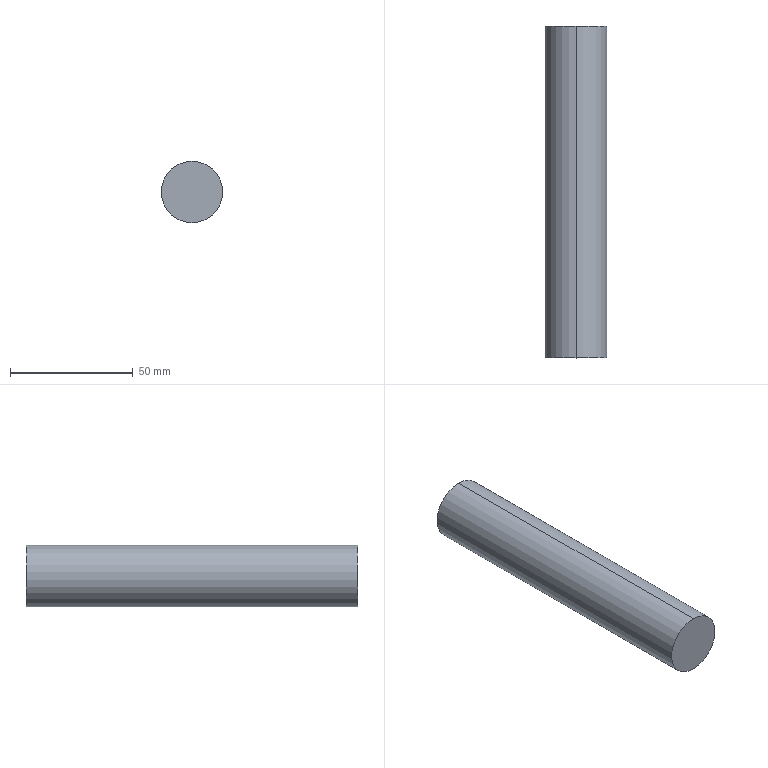Part | 1 solid | 4 faces | box 25 x 135 x 25 mm | volume 66268 mm3 | plane 2 | cylinder 2 | commonest cylinder face diameters 25 x2
STEP:
#1=CARTESIAN_POINT('',(0.,0.,0.));
#2=DIRECTION('',(0.,0.,1.));
#3=DIRECTION('',(1.,0.,0.));
#4=AXIS2_PLACEMENT_3D('',#1,#2,#3);
#5=CARTESIAN_POINT('',(-239.028,-100.5,-288.05));
#6=VERTEX_POINT('',#5);
#7=CARTESIAN_POINT('',(-239.028,-100.5,-313.05));
#8=VERTEX_POINT('',#7);
#9=CARTESIAN_POINT('',(-239.028,-100.5,-300.55));
#10=DIRECTION('',(0.,1.,0.));
#11=DIRECTION('',(0.,0.,-1.));
#12=AXIS2_PLACEMENT_3D('',#9,#10,#11);
#13=CIRCLE('',#12,12.5);
#14=CARTESIAN_POINT('',(-239.028,-100.5,-300.55));
#15=DIRECTION('',(0.,1.,0.));
#16=DIRECTION('',(0.,0.,1.));
#17=AXIS2_PLACEMENT_3D('',#14,#15,#16);
#18=PLANE('',#17);
#19=CARTESIAN_POINT('',(0.,0.));
#20=DIRECTION('',(-1.,0.));
#21=AXIS2_PLACEMENT_2D('',#19,#20);
#22=CIRCLE('',#21,12.5);
#23=(GEOMETRIC_REPRESENTATION_CONTEXT(2)PARAMETRIC_REPRESENTATION_CONTEXT()REPRESENTATION_CONTEXT('',''));
#24=DEFINITIONAL_REPRESENTATION('',(#22),#23);
#25=PCURVE('',#18,#24);
#26=CARTESIAN_POINT('',(-239.028,254.5,-300.55));
#27=DIRECTION('',(0.,-1.,0.));
#28=DIRECTION('',(-1.,0.,0.));
#29=AXIS2_PLACEMENT_3D('',#26,#27,#28);
#30=CYLINDRICAL_SURFACE('',#29,12.5);
#31=CARTESIAN_POINT('',(7.854,355.));
#32=DIRECTION('',(-1.,0.));
#33=VECTOR('',#32,1.);
#34=LINE('',#31,#33);
#35=(GEOMETRIC_REPRESENTATION_CONTEXT(2)PARAMETRIC_REPRESENTATION_CONTEXT()REPRESENTATION_CONTEXT('',''));
#36=DEFINITIONAL_REPRESENTATION('',(#34),#35);
#37=PCURVE('',#30,#36);
#38=SURFACE_CURVE('',#13,(#25,#37),.PCURVE_S1.);
#39=EDGE_CURVE('',#6,#8,#38,.T.);
#40=ORIENTED_EDGE('',*,*,#39,.F.);
#41=CARTESIAN_POINT('',(-239.028,-100.5,-300.55));
#42=DIRECTION('',(0.,1.,0.));
#43=DIRECTION('',(0.,0.,-1.));
#44=AXIS2_PLACEMENT_3D('',#41,#42,#43);
#45=CIRCLE('',#44,12.5);
#46=CARTESIAN_POINT('',(0.,0.));
#47=DIRECTION('',(-1.,0.));
#48=AXIS2_PLACEMENT_2D('',#46,#47);
#49=CIRCLE('',#48,12.5);
#50=(GEOMETRIC_REPRESENTATION_CONTEXT(2)PARAMETRIC_REPRESENTATION_CONTEXT()REPRESENTATION_CONTEXT('',''));
#51=DEFINITIONAL_REPRESENTATION('',(#49),#50);
#52=PCURVE('',#18,#51);
#53=CARTESIAN_POINT('',(-239.028,254.5,-300.55));
#54=DIRECTION('',(0.,-1.,0.));
#55=DIRECTION('',(1.,0.,0.));
#56=AXIS2_PLACEMENT_3D('',#53,#54,#55);
#57=CYLINDRICAL_SURFACE('',#56,12.5);
#58=CARTESIAN_POINT('',(4.712,355.));
#59=DIRECTION('',(-1.,0.));
#60=VECTOR('',#59,1.);
#61=LINE('',#58,#60);
#62=(GEOMETRIC_REPRESENTATION_CONTEXT(2)PARAMETRIC_REPRESENTATION_CONTEXT()REPRESENTATION_CONTEXT('',''));
#63=DEFINITIONAL_REPRESENTATION('',(#61),#62);
#64=PCURVE('',#57,#63);
#65=SURFACE_CURVE('',#45,(#52,#64),.PCURVE_S1.);
#66=EDGE_CURVE('',#8,#6,#65,.T.);
#67=ORIENTED_EDGE('',*,*,#66,.F.);
#68=EDGE_LOOP('',(#40,#67));
#69=FACE_BOUND('',#68,.T.);
#70=ADVANCED_FACE('',(#69),#18,.F.);
#71=CARTESIAN_POINT('',(-239.028,34.5,-288.05));
#72=VERTEX_POINT('',#71);
#73=CARTESIAN_POINT('',(-239.028,34.5,-288.05));
#74=DIRECTION('',(0.,-1.,0.));
#75=VECTOR('',#74,1.);
#76=LINE('',#73,#75);
#77=CARTESIAN_POINT('',(1.571,220.));
#78=DIRECTION('',(0.,1.));
#79=VECTOR('',#78,1.);
#80=LINE('',#77,#79);
#81=(GEOMETRIC_REPRESENTATION_CONTEXT(2)PARAMETRIC_REPRESENTATION_CONTEXT()REPRESENTATION_CONTEXT('',''));
#82=DEFINITIONAL_REPRESENTATION('',(#80),#81);
#83=PCURVE('',#57,#82);
#84=CARTESIAN_POINT('',(4.712,220.));
#85=DIRECTION('',(0.,1.));
#86=VECTOR('',#85,1.);
#87=LINE('',#84,#86);
#88=(GEOMETRIC_REPRESENTATION_CONTEXT(2)PARAMETRIC_REPRESENTATION_CONTEXT()REPRESENTATION_CONTEXT('',''));
#89=DEFINITIONAL_REPRESENTATION('',(#87),#88);
#90=PCURVE('',#30,#89);
#91=SURFACE_CURVE('',#76,(#83,#90),.PCURVE_S1.);
#92=EDGE_CURVE('',#72,#6,#91,.T.);
#93=ORIENTED_EDGE('',*,*,#92,.F.);
#94=CARTESIAN_POINT('',(-239.028,34.5,-313.05));
#95=VERTEX_POINT('',#94);
#96=CARTESIAN_POINT('',(-239.028,34.5,-300.55));
#97=DIRECTION('',(0.,1.,0.));
#98=DIRECTION('',(0.,0.,-1.));
#99=AXIS2_PLACEMENT_3D('',#96,#97,#98);
#100=CIRCLE('',#99,12.5);
#101=CARTESIAN_POINT('',(4.712,220.));
#102=DIRECTION('',(-1.,0.));
#103=VECTOR('',#102,1.);
#104=LINE('',#101,#103);
#105=(GEOMETRIC_REPRESENTATION_CONTEXT(2)PARAMETRIC_REPRESENTATION_CONTEXT()REPRESENTATION_CONTEXT('',''));
#106=DEFINITIONAL_REPRESENTATION('',(#104),#105);
#107=PCURVE('',#57,#106);
#108=CARTESIAN_POINT('',(-254.,34.5,-299.55));
#109=DIRECTION('',(0.,-1.,0.));
#110=DIRECTION('',(0.,0.,-1.));
#111=AXIS2_PLACEMENT_3D('',#108,#109,#110);
#112=PLANE('',#111);
#113=CARTESIAN_POINT('',(13.5,14.972));
#114=CARTESIAN_POINT('',(13.5,-6.678));
#115=CARTESIAN_POINT('',(-5.25,4.147));
#116=CARTESIAN_POINT('',(-24.,14.972));
#117=CARTESIAN_POINT('',(-5.25,25.798));
#118=CARTESIAN_POINT('',(13.5,36.623));
#119=CARTESIAN_POINT('',(13.5,14.972));
#120=(BOUNDED_CURVE()B_SPLINE_CURVE(2,(#113,#114,#115,#116,#117,#118,#119),.UNSPECIFIED.,.T.,.F.)B_SPLINE_CURVE_WITH_KNOTS((1,2,2,2,2,1),(-2.094,0.,2.094,4.189,6.283,8.378),.UNSPECIFIED.)CURVE()GEOMETRIC_REPRESENTATION_ITEM()RATIONAL_B_SPLINE_CURVE((1.,0.5,1.,0.5,1.,0.5,1.))REPRESENTATION_ITEM(''));
#121=(GEOMETRIC_REPRESENTATION_CONTEXT(2)PARAMETRIC_REPRESENTATION_CONTEXT()REPRESENTATION_CONTEXT('',''));
#122=DEFINITIONAL_REPRESENTATION('',(#120),#121);
#123=PCURVE('',#112,#122);
#124=SURFACE_CURVE('',#100,(#107,#123),.PCURVE_S1.);
#125=EDGE_CURVE('',#95,#72,#124,.T.);
#126=ORIENTED_EDGE('',*,*,#125,.F.);
#127=CARTESIAN_POINT('',(-239.028,34.5,-313.05));
#128=DIRECTION('',(0.,-1.,0.));
#129=VECTOR('',#128,1.);
#130=LINE('',#127,#129);
#131=CARTESIAN_POINT('',(4.712,220.));
#132=DIRECTION('',(0.,1.));
#133=VECTOR('',#132,1.);
#134=LINE('',#131,#133);
#135=(GEOMETRIC_REPRESENTATION_CONTEXT(2)PARAMETRIC_REPRESENTATION_CONTEXT()REPRESENTATION_CONTEXT('',''));
#136=DEFINITIONAL_REPRESENTATION('',(#134),#135);
#137=PCURVE('',#57,#136);
#138=CARTESIAN_POINT('',(1.571,220.));
#139=DIRECTION('',(0.,1.));
#140=VECTOR('',#139,1.);
#141=LINE('',#138,#140);
#142=(GEOMETRIC_REPRESENTATION_CONTEXT(2)PARAMETRIC_REPRESENTATION_CONTEXT()REPRESENTATION_CONTEXT('',''));
#143=DEFINITIONAL_REPRESENTATION('',(#141),#142);
#144=PCURVE('',#30,#143);
#145=SURFACE_CURVE('',#130,(#137,#144),.PCURVE_S1.);
#146=EDGE_CURVE('',#95,#8,#145,.T.);
#147=ORIENTED_EDGE('',*,*,#146,.T.);
#148=ORIENTED_EDGE('',*,*,#66,.T.);
#149=EDGE_LOOP('',(#93,#126,#147,#148));
#150=FACE_BOUND('',#149,.T.);
#151=ADVANCED_FACE('',(#150),#57,.T.);
#152=ORIENTED_EDGE('',*,*,#125,.T.);
#153=CARTESIAN_POINT('',(-239.028,34.5,-300.55));
#154=DIRECTION('',(0.,1.,0.));
#155=DIRECTION('',(0.,0.,-1.));
#156=AXIS2_PLACEMENT_3D('',#153,#154,#155);
#157=CIRCLE('',#156,12.5);
#158=CARTESIAN_POINT('',(13.5,14.972));
#159=CARTESIAN_POINT('',(13.5,-6.678));
#160=CARTESIAN_POINT('',(-5.25,4.147));
#161=CARTESIAN_POINT('',(-24.,14.972));
#162=CARTESIAN_POINT('',(-5.25,25.798));
#163=CARTESIAN_POINT('',(13.5,36.623));
#164=CARTESIAN_POINT('',(13.5,14.972));
#165=(BOUNDED_CURVE()B_SPLINE_CURVE(2,(#158,#159,#160,#161,#162,#163,#164),.UNSPECIFIED.,.T.,.F.)B_SPLINE_CURVE_WITH_KNOTS((1,2,2,2,2,1),(-2.094,0.,2.094,4.189,6.283,8.378),.UNSPECIFIED.)CURVE()GEOMETRIC_REPRESENTATION_ITEM()RATIONAL_B_SPLINE_CURVE((1.,0.5,1.,0.5,1.,0.5,1.))REPRESENTATION_ITEM(''));
#166=(GEOMETRIC_REPRESENTATION_CONTEXT(2)PARAMETRIC_REPRESENTATION_CONTEXT()REPRESENTATION_CONTEXT('',''));
#167=DEFINITIONAL_REPRESENTATION('',(#165),#166);
#168=PCURVE('',#112,#167);
#169=CARTESIAN_POINT('',(7.854,220.));
#170=DIRECTION('',(-1.,0.));
#171=VECTOR('',#170,1.);
#172=LINE('',#169,#171);
#173=(GEOMETRIC_REPRESENTATION_CONTEXT(2)PARAMETRIC_REPRESENTATION_CONTEXT()REPRESENTATION_CONTEXT('',''));
#174=DEFINITIONAL_REPRESENTATION('',(#172),#173);
#175=PCURVE('',#30,#174);
#176=SURFACE_CURVE('',#157,(#168,#175),.PCURVE_S1.);
#177=EDGE_CURVE('',#72,#95,#176,.T.);
#178=ORIENTED_EDGE('',*,*,#177,.T.);
#179=EDGE_LOOP('',(#152,#178));
#180=FACE_BOUND('',#179,.T.);
#181=ADVANCED_FACE('',(#180),#112,.F.);
#182=ORIENTED_EDGE('',*,*,#92,.T.);
#183=ORIENTED_EDGE('',*,*,#39,.T.);
#184=ORIENTED_EDGE('',*,*,#146,.F.);
#185=ORIENTED_EDGE('',*,*,#177,.F.);
#186=EDGE_LOOP('',(#182,#183,#184,#185));
#187=FACE_BOUND('',#186,.T.);
#188=ADVANCED_FACE('',(#187),#30,.T.);
#189=CLOSED_SHELL('',(#70,#151,#181,#188));
#190=MANIFOLD_SOLID_BREP('',#189);
#191=(LENGTH_UNIT()NAMED_UNIT(*)SI_UNIT(.MILLI.,.METRE.));
#192=UNCERTAINTY_MEASURE_WITH_UNIT(LENGTH_MEASURE(0.0000001),#191,'','');
#193=(NAMED_UNIT(*)PLANE_ANGLE_UNIT()SI_UNIT($,.RADIAN.));
#194=(NAMED_UNIT(*)SI_UNIT($,.STERADIAN.)SOLID_ANGLE_UNIT());
#195=(GEOMETRIC_REPRESENTATION_CONTEXT(3)GLOBAL_UNCERTAINTY_ASSIGNED_CONTEXT((#192))GLOBAL_UNIT_ASSIGNED_CONTEXT((#191,#193,#194))REPRESENTATION_CONTEXT('',''));
#196=ADVANCED_BREP_SHAPE_REPRESENTATION('',(#4,#190),#195);